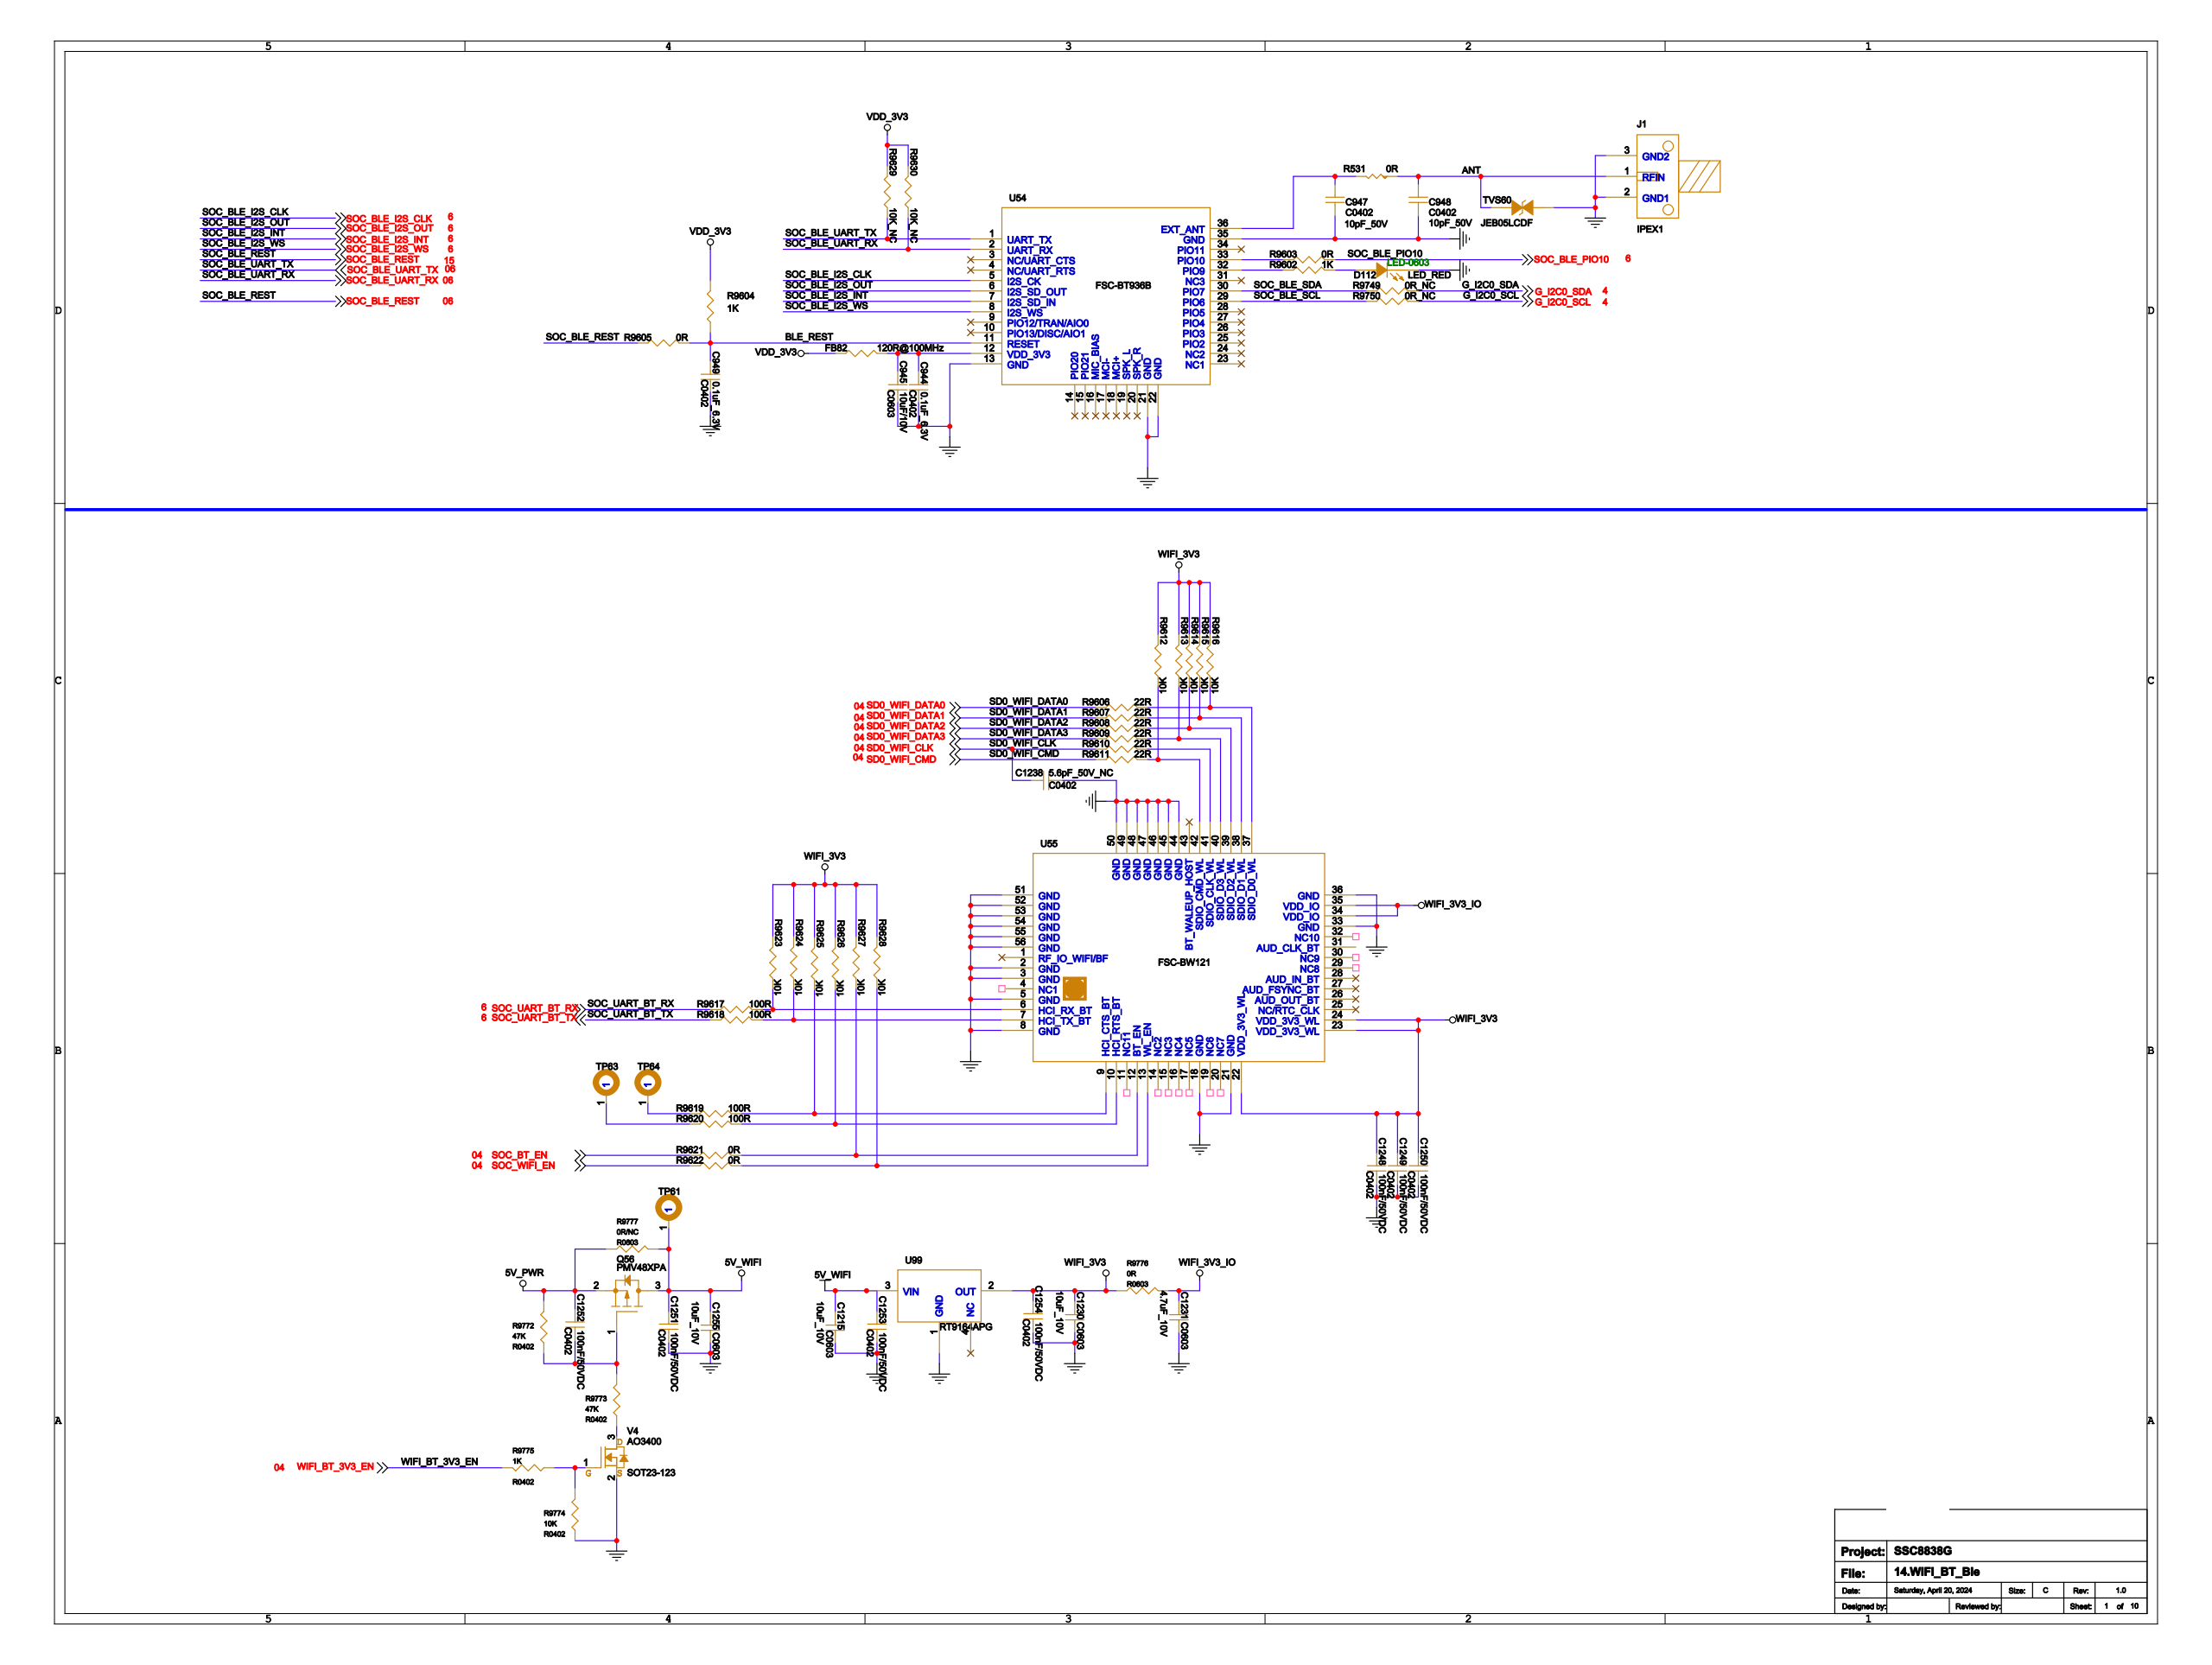Circuit board | Cadence Allegro | 958 parts | 601 nets | one sheet of the schematic
Parts on this sheet (reference | value | footprint):
C944 | 0.1uF_6.3V | C0402
C945 | 10uF/10V | C0603
C947 | 10pF_50V | C0402
C948 | 10pF_50V | C0402
C949 | 0.1uF_6.3V | C0402
C1215 | 10uF_10V | C0603
C1230 | 10uF_10V | C0603
C1231 | 4.7uF_10V | C0603
C1238 | 5.6pF_50V_NC | C0402
C1248 | 100nF/50VDC | C0402
C1249 | 100nF/50VDC | C0402
C1250 | 100nF/50VDC | C0402
C1251 | 100nF/50VDC | C0402
C1252 | 100nF/50VDC | C0402
C1253 | 100nF/50VDC | C0402
C1254 | 100nF/50VDC | C0402
C1255 | 10uF_10V | C0603
D112 | LED_RED | LED-0603
FB82 | 120R@100MHz | R0402
J1 | IPEX1 | RF_3X3_1H1_25
Q56 | PMV48XPA | SOT-23
R531 | 0R | R0402
R9602 | 1K | R0402
R9603 | 0R | R0402
R9604 | 1K | R0402
R9605 | 0R | R0402
R9606 | 22R | R0402
R9607 | 22R | R0402
R9608 | 22R | R0402
R9609 | 22R | R0402
R9610 | 22R | R0402
R9611 | 22R | R0402
R9612 | 10K | R0402
R9613 | 10K | R0402
R9614 | 10K | R0402
R9615 | 10K | R0402
R9616 | 10K | R0402
R9617 | 100R | R0402
R9618 | 100R | R0402
R9619 | 100R | R0402
R9620 | 100R | R0402
R9621 | 0R | R0402
R9622 | 0R | R0402
R9623 | 10K | R0402
R9624 | 10K | R0402
R9625 | 10K | R0402
R9626 | 10K | R0402
R9627 | 10K | R0402
R9628 | 10K | R0402
R9629 | 10K_NC | R0402
R9630 | 10K_NC | R0402
R9749 | 0R_NC | R0402
R9750 | 0R_NC | R0402
R9772 | 47K | R0402
R9773 | 47K | R0402
R9774 | 10K | R0402
R9775 | 1K | R0402
R9776 | 0R | R0603
R9777 | 0R/NC | R0603
TP61 | HOLE | TP_0R50
TP63 | HOLE | TP_0R50
TP64 | HOLE | TP_0R50
TVS60 | JEB05LCDF | R0402
U54 | FSC-BT936B | FSC_BT936
U55 | FSC-BW121 | FSC_121_56PIN
U99 | RT9164APG | SOT-223-3
V4 | AO3400 | SOT23-123
Nets of these parts (net: part-pin ...):
GND: C944-1 C945-1 C947-2 C948-2 C949-1 C1215-1 C1230-1 C1231-1 C1238-2 C1248-2 C1249-2 C1250-2 C1251-2 C1253-2 C1254-2 C1255-1 D112-2 J1-2 J1-3 R9774-1 TVS60-1 U54-13 U54-21 U54-22 U54-35 U99-1 V4-2 U55-2 U55-3 U55-5 U55-8 U55-18 U55-21 U55-33 U55-36 U55-44 U55-45 U55-46 U55-47 U55-48 U55-49 U55-50 U55-51 U55-52 U55-53 U55-54 U55-55 U55-56
5V_PWR: C1252-1 Q56-2 R9772-2 R9777-1
3V3_NORMAL: FB82-1 R9604-1 R9629-1 R9630-1
WIFI_3V3: C1230-2 C1248-1 C1249-1 C1250-1 C1254-1 R9612-1 R9613-1 R9614-1 R9615-1 R9616-1 R9623-1 R9624-1 R9625-1 R9626-1 R9627-1 R9628-1 R9776-1 U99-2 U55-22 U55-23 U55-24
5V_WIFI: C1215-2 C1251-1 C1253-1 C1255-2 Q56-3 R9777-2 TP61-1 U99-3
N21504244: C1252-2 Q56-1 R9772-1 R9773-2
N21211255: C944-2 C945-2 FB82-2 U54-12
WIFI_3V3_IO: C1231-2 R9776-2 U55-34 U55-35
SD0_WIFI_CLK: C1238-1 R9610-2
BLE_REST: C949-2 R9604-2 R9605-1 U54-11
N21212523: C947-1 R531-2 U54-36
ANT: C948-1 J1-1 R531-1 TVS60-2
N21212305: D112-1 R9602-1
N21216089: R9617-1 R9623-2 U55-6
SOC_UART_BT_RX: R9617-2
N21216090: R9618-1 R9624-2 U55-7
SOC_UART_BT_TX: R9618-2
N21216154: R9619-1 R9625-2 U55-9
N22112784: R9619-2 TP64-1
N21216156: R9620-1 R9626-2 U55-10
N22112789: R9620-2 TP63-1
N21215035: R9611-1 R9612-2 U55-42
N21215097: R9609-1 R9613-2 U55-40
N21215107: R9608-1 R9614-2 U55-39
N21215117: R9607-1 R9615-2 U55-38
N21215119: R9606-1 R9616-2 U55-37
N21216280: R9621-1 R9627-2 U55-12
N21216282: R9622-1 R9628-2 U55-13
G_I2C0_SCL: R9750-1
G_I2C0_SDA: R9749-1
N21504284: R9774-2 R9775-1 V4-1
SOC_BLE_PIO10: R9603-1
N21745612: R9603-2 U54-33
SOC_BLE_REST: R9605-2
SOC_BT_EN: R9621-2
SOC_WIFI_EN: R9622-2
N21744746: R9602-2 U54-32
SD0_WIFI_DATA0: R9606-2
SD0_WIFI_DATA1: R9607-2
SD0_WIFI_DATA2: R9608-2
SD0_WIFI_DATA3: R9609-2
N21215060: R9610-1 U55-41
SD0_WIFI_CMD: R9611-2
SOC_BLE_UART_TX: R9629-2 U54-1
SOC_BLE_UART_RX: R9630-2 U54-2
SOC_BLE_SDA: R9749-2 U54-30
SOC_BLE_SCL: R9750-2 U54-29
N21504248: R9773-1 V4-3
WIFI_BT_3V3_EN: R9775-2
SOC_BLE_I2S_WS: U54-8
SOC_BLE_I2S_OUT: U54-6
SOC_BLE_I2S_INT: U54-7
SOC_BLE_I2S_CLK: U54-5
AUD_CLK_BT: U55-31